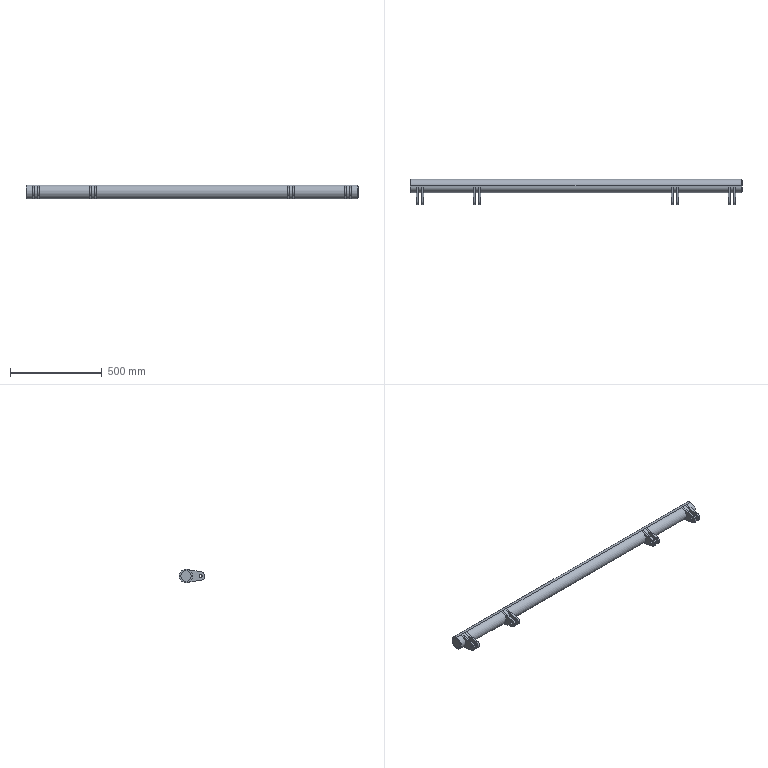Part | SolidWorks | features ICE 3, LPattern 2, MirrorSolid 2, HoleWzd 1, WeldMemberFeat 1, WeldmentFeature 1 | 11 solids | 78 faces | box 1806 x 139 x 73 mm | volume 3217271 mm3 | cylinder 40 | plane 38 | commonest cylinder face diameters 16.5 x16 45 x8 73.111 x8 57 x6 73 x2